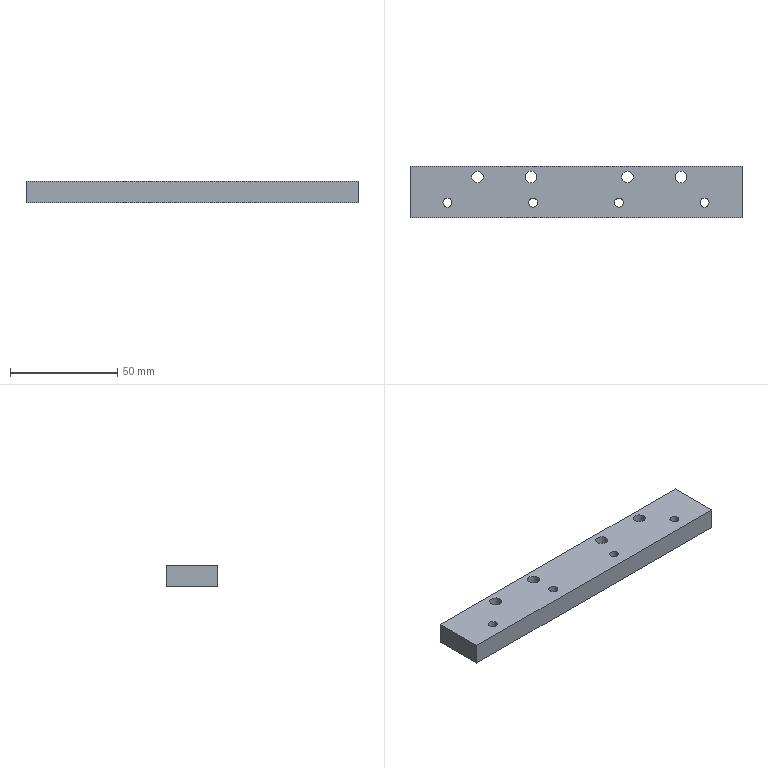Part | STEP file | 0232_209_Plate | 1 solid | 22 faces | box 155 x 24 x 10 mm | volume 35695 mm3 | cylinder 16 | plane 6 | commonest cylinder face diameters 4.2 x8 5.5 x8